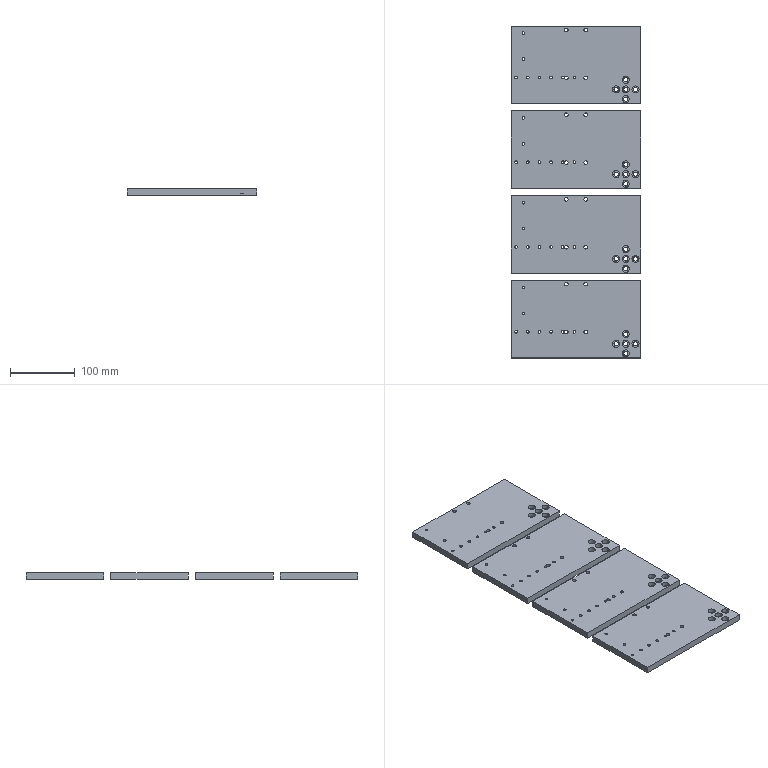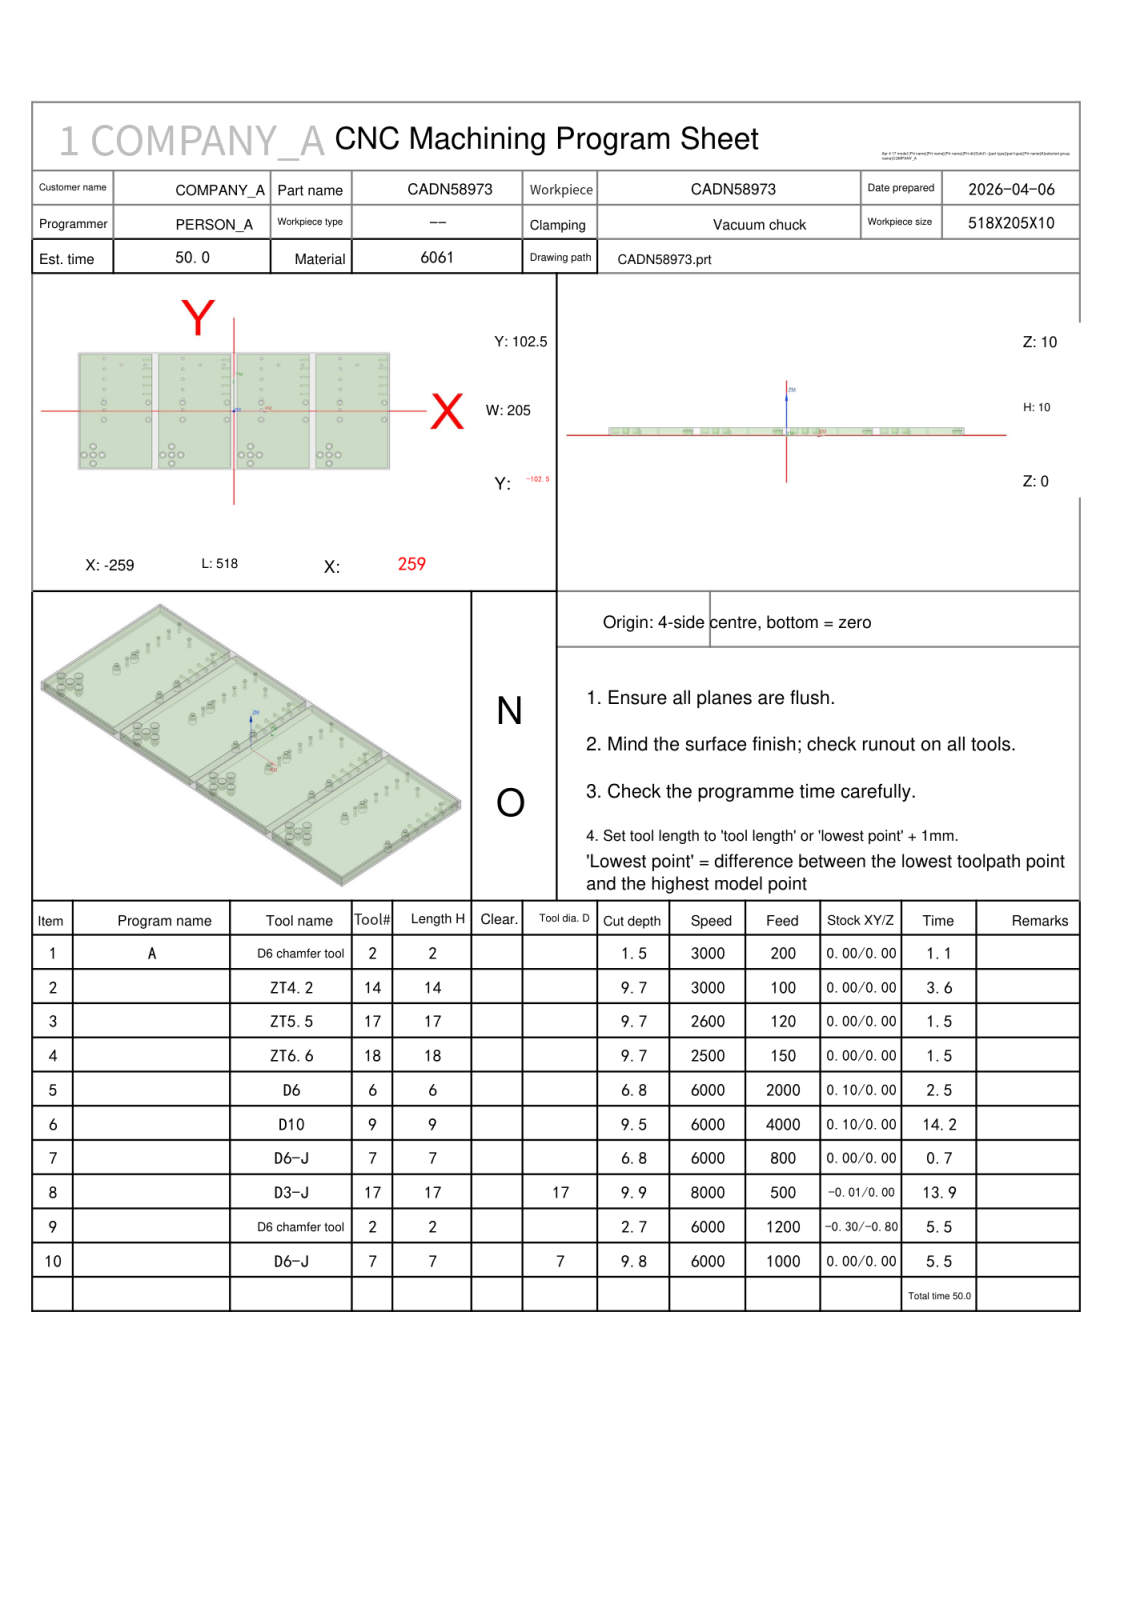NC program | NX | posted by the shop | part box 200 x 513 x 10 mm
Lines 9278 to 10035 of 10035:
N9 T02 M06
(D6 chamfer tool  D=6. R=0. H=02 ce=0.00 di=0.00)
G00 G90 G54 X258.628 Y.25 M03 S6000
G43 H02 Z30.
M08
Z12.099
G01 Z8.5 F1200.
G03 X258.328 Y.33 I-.3 J-.52
X257.808 Y.03 I0.0 J-.6
G01 X257.8 Y0.0
Y-100.
G02 X256.5 Y-101.3 I-1.3 J0.0
G01 X136.5
G02 X135.2 Y-100. I0.0 J1.3
G01 Y100.
G02 X136.5 Y101.3 I1.3 J0.0
G01 X256.5
G02 X257.8 Y100. I0.0 J-1.3
G01 Y0.0
X257.808 Y-.03
G03 X258.328 Y-.33 I.52 J.3
X258.628 Y-.25 I0.0 J.6
G01 Z12.099
G00 Z30.
X127.628 Y.25
Z12.099
G01 Z8.5
G03 X127.328 Y.33 I-.3 J-.52
X126.808 Y.03 I0.0 J-.6
G01 X126.8 Y0.0
Y-100.
G02 X125.5 Y-101.3 I-1.3 J0.0
G01 X5.5
G02 X4.2 Y-100. I0.0 J1.3
G01 Y100.
G02 X5.5 Y101.3 I1.3 J0.0
G01 X125.5
G02 X126.8 Y100. I0.0 J-1.3
G01 Y0.0
X126.808 Y-.03
G03 X127.328 Y-.33 I.52 J.3
X127.628 Y-.25 I0.0 J.6
G01 Z12.099
G00 Z30.
X-3.372 Y.25
Z12.099
G01 Z8.5
G03 X-3.672 Y.33 I-.3 J-.52
X-4.192 Y.03 I0.0 J-.6
G01 X-4.2 Y0.0
Y-100.
G02 X-5.5 Y-101.3 I-1.3 J0.0
G01 X-125.5
G02 X-126.8 Y-100. I0.0 J1.3
G01 Y100.
G02 X-125.5 Y101.3 I1.3 J0.0
G01 X-5.5
G02 X-4.2 Y100. I0.0 J-1.3
G01 Y0.0
X-4.192 Y-.03
G03 X-3.672 Y-.33 I.52 J.3
X-3.372 Y-.25 I0.0 J.6
G01 Z12.099
G00 Z30.
X-134.372 Y.25
Z12.099
G01 Z8.5
G03 X-134.672 Y.33 I-.3 J-.52
X-135.192 Y.03 I0.0 J-.6
G01 X-135.2 Y0.0
Y-100.
G02 X-136.5 Y-101.3 I-1.3 J0.0
G01 X-256.5
G02 X-257.8 Y-100. I0.0 J1.3
G01 Y100.
G02 X-256.5 Y101.3 I1.3 J0.0
G01 X-136.5
G02 X-135.2 Y100. I0.0 J-1.3
G01 Y0.0
X-135.192 Y-.03
G03 X-134.672 Y-.33 I.52 J.3
X-134.372 Y-.25 I0.0 J.6
G01 Z12.099
G00 Z30.
G00 G90 X-216. Y2.515 M03 S5000
Z30.
G98 G81 X-216. Y2.515 Z7.333 R13. F150.
Y20.515
Y38.515
Y56.515
Y74.515
Y92.515
X-187.5 Y81.264
X-147.5
X-85. Y2.515
Y20.515
Y38.515
Y56.515
Y74.515
Y92.515
X-56.5 Y81.264
X-16.5
X46. Y2.515
Y20.515
Y38.515
Y56.515
Y74.515
Y92.515
X74.5 Y81.264
X114.5
X177. Y92.515
X245.5 Y81.264
X205.5
X177. Y74.515
Y56.515
Y38.515
Y20.515
Y2.515
G80
G00 Z30.
G00 G90 X249.853 Y-15.065 M03 S6000
Z30.
Z9.1
G01 Z8.6 F600.
X249. Y-15.15
G03 X250.5 Y-16.65 I1.5 J0.0
X252.15 Y-15. I0.0 J1.65
X250.5 Y-13.35 I-1.65 J0.0
X248.85 Y-15. I0.0 J-1.65
X250.5 Y-16.65 I1.65 J0.0
X252. Y-15.15 I0.0 J1.5
G01 X251.147 Y-15.065
Z9.1
G00 Z30.
X249.853 Y14.935
Z9.1
G01 Z8.6
X249. Y14.85
G03 X250.5 Y13.35 I1.5 J0.0
X252.15 Y15. I0.0 J1.65
X250.5 Y16.65 I-1.65 J0.0
X248.85 Y15. I0.0 J-1.65
X250.5 Y13.35 I1.65 J0.0
X252. Y14.85 I0.0 J1.5
G01 X251.147 Y14.935
Z9.1
G00 Z30.
X175.853
Z9.1
G01 Z8.6
X175. Y14.85
G03 X176.5 Y13.35 I1.5 J0.0
X178.15 Y15. I0.0 J1.65
X176.5 Y16.65 I-1.65 J0.0
X174.85 Y15. I0.0 J-1.65
X176.5 Y13.35 I1.65 J0.0
X178. Y14.85 I0.0 J1.5
G01 X177.147 Y14.935
Z9.1
G00 Z30.
X175.853 Y-15.065
Z9.1
G01 Z8.6
X175. Y-15.15
G03 X176.5 Y-16.65 I1.5 J0.0
X178.15 Y-15. I0.0 J1.65
X176.5 Y-13.35 I-1.65 J0.0
X174.85 Y-15. I0.0 J-1.65
X176.5 Y-16.65 I1.65 J0.0
X178. Y-15.15 I0.0 J1.5
G01 X177.147 Y-15.065
Z9.1
G00 Z30.
X118.853
Z9.1
G01 Z8.6
X118. Y-15.15
G03 X119.5 Y-16.65 I1.5 J0.0
X121.15 Y-15. I0.0 J1.65
X119.5 Y-13.35 I-1.65 J0.0
X117.85 Y-15. I0.0 J-1.65
X119.5 Y-16.65 I1.65 J0.0
X121. Y-15.15 I0.0 J1.5
G01 X120.147 Y-15.065
Z9.1
G00 Z30.
X118.853 Y14.935
Z9.1
G01 Z8.6
X118. Y14.85
G03 X119.5 Y13.35 I1.5 J0.0
X121.15 Y15. I0.0 J1.65
X119.5 Y16.65 I-1.65 J0.0
X117.85 Y15. I0.0 J-1.65
X119.5 Y13.35 I1.65 J0.0
X121. Y14.85 I0.0 J1.5
G01 X120.147 Y14.935
Z9.1
G00 Z30.
X44.853
Z9.1
G01 Z8.6
X44. Y14.85
G03 X45.5 Y13.35 I1.5 J0.0
X47.15 Y15. I0.0 J1.65
X45.5 Y16.65 I-1.65 J0.0
X43.85 Y15. I0.0 J-1.65
X45.5 Y13.35 I1.65 J0.0
X47. Y14.85 I0.0 J1.5
G01 X46.147 Y14.935
Z9.1
G00 Z30.
X44.853 Y-15.065
Z9.1
G01 Z8.6
X44. Y-15.15
G03 X45.5 Y-16.65 I1.5 J0.0
X47.15 Y-15. I0.0 J1.65
X45.5 Y-13.35 I-1.65 J0.0
X43.85 Y-15. I0.0 J-1.65
X45.5 Y-16.65 I1.65 J0.0
X47. Y-15.15 I0.0 J1.5
G01 X46.147 Y-15.065
Z9.1
G00 Z30.
X-12.147
Z9.1
G01 Z8.6
X-13. Y-15.15
G03 X-11.5 Y-16.65 I1.5 J0.0
X-9.85 Y-15. I0.0 J1.65
X-11.5 Y-13.35 I-1.65 J0.0
X-13.15 Y-15. I0.0 J-1.65
X-11.5 Y-16.65 I1.65 J0.0
X-10. Y-15.15 I0.0 J1.5
G01 X-10.853 Y-15.065
Z9.1
G00 Z30.
X-12.147 Y14.935
Z9.1
G01 Z8.6
X-13. Y14.85
G03 X-11.5 Y13.35 I1.5 J0.0
X-9.85 Y15. I0.0 J1.65
X-11.5 Y16.65 I-1.65 J0.0
X-13.15 Y15. I0.0 J-1.65
X-11.5 Y13.35 I1.65 J0.0
X-10. Y14.85 I0.0 J1.5
G01 X-10.853 Y14.935
Z9.1
G00 Z30.
X-86.147
Z9.1
G01 Z8.6
X-87. Y14.85
G03 X-85.5 Y13.35 I1.5 J0.0
X-83.85 Y15. I0.0 J1.65
X-85.5 Y16.65 I-1.65 J0.0
X-87.15 Y15. I0.0 J-1.65
X-85.5 Y13.35 I1.65 J0.0
X-84. Y14.85 I0.0 J1.5
G01 X-84.853 Y14.935
Z9.1
G00 Z30.
X-86.147 Y-15.065
Z9.1
G01 Z8.6
X-87. Y-15.15
G03 X-85.5 Y-16.65 I1.5 J0.0
X-83.85 Y-15. I0.0 J1.65
X-85.5 Y-13.35 I-1.65 J0.0
X-87.15 Y-15. I0.0 J-1.65
X-85.5 Y-16.65 I1.65 J0.0
X-84. Y-15.15 I0.0 J1.5
G01 X-84.853 Y-15.065
Z9.1
G00 Z30.
X-143.147
Z9.1
G01 Z8.6
X-144. Y-15.15
G03 X-142.5 Y-16.65 I1.5 J0.0
X-140.85 Y-15. I0.0 J1.65
X-142.5 Y-13.35 I-1.65 J0.0
X-144.15 Y-15. I0.0 J-1.65
X-142.5 Y-16.65 I1.65 J0.0
X-141. Y-15.15 I0.0 J1.5
G01 X-141.853 Y-15.065
Z9.1
G00 Z30.
X-143.147 Y14.935
Z9.1
G01 Z8.6
X-144. Y14.85
G03 X-142.5 Y13.35 I1.5 J0.0
X-140.85 Y15. I0.0 J1.65
X-142.5 Y16.65 I-1.65 J0.0
X-144.15 Y15. I0.0 J-1.65
X-142.5 Y13.35 I1.65 J0.0
X-141. Y14.85 I0.0 J1.5
G01 X-141.853 Y14.935
Z9.1
G00 Z30.
X-217.147
Z9.1
G01 Z8.6
X-218. Y14.85
G03 X-216.5 Y13.35 I1.5 J0.0
X-214.85 Y15. I0.0 J1.65
X-216.5 Y16.65 I-1.65 J0.0
X-218.15 Y15. I0.0 J-1.65
X-216.5 Y13.35 I1.65 J0.0
X-215. Y14.85 I0.0 J1.5
G01 X-215.853 Y14.935
Z9.1
G00 Z30.
X-217.147 Y-15.065
Z9.1
G01 Z8.6
X-218. Y-15.15
G03 X-216.5 Y-16.65 I1.5 J0.0
X-214.85 Y-15. I0.0 J1.65
X-216.5 Y-13.35 I-1.65 J0.0
X-218.15 Y-15. I0.0 J-1.65
X-216.5 Y-16.65 I1.65 J0.0
X-215. Y-15.15 I0.0 J1.5
G01 X-215.853 Y-15.065
Z9.1
G00 Z30.
G00 G90 X170.795 Y-77.721 M03 S6000
Z30.
Z8.5
G01 Z8. F600.
X170.5 Y-77.8
G03 X173.5 Y-80.8 I3. J0.0
X177.3 Y-77. I0.0 J3.8
X173.5 Y-73.2 I-3.8 J0.0
X169.7 Y-77. I0.0 J-3.8
X173.5 Y-80.8 I3.8 J0.0
X176.5 Y-77.8 I0.0 J3.
G01 X176.205 Y-77.721
Z8.5
G00 Z30.
X155.795 Y-62.721
Z8.5
G01 Z8.
X155.5 Y-62.8
G03 X158.5 Y-65.8 I3. J0.0
X162.3 Y-62. I0.0 J3.8
X158.5 Y-58.2 I-3.8 J0.0
X154.7 Y-62. I0.0 J-3.8
X158.5 Y-65.8 I3.8 J0.0
X161.5 Y-62.8 I0.0 J3.
G01 X161.205 Y-62.721
Z8.5
G00 Z30.
X155.795 Y-77.721
Z8.5
G01 Z8.
X155.5 Y-77.8
G03 X158.5 Y-80.8 I3. J0.0
X162.3 Y-77. I0.0 J3.8
X158.5 Y-73.2 I-3.8 J0.0
X154.7 Y-77. I0.0 J-3.8
X158.5 Y-80.8 I3.8 J0.0
X161.5 Y-77.8 I0.0 J3.
G01 X161.205 Y-77.721
Z8.5
G00 Z30.
X155.795 Y-92.721
Z8.5
G01 Z8.
X155.5 Y-92.8
G03 X158.5 Y-95.8 I3. J0.0
X162.3 Y-92. I0.0 J3.8
X158.5 Y-88.2 I-3.8 J0.0
X154.7 Y-92. I0.0 J-3.8
X158.5 Y-95.8 I3.8 J0.0
X161.5 Y-92.8 I0.0 J3.
G01 X161.205 Y-92.721
Z8.5
G00 Z30.
X140.795 Y-77.721
Z8.5
G01 Z8.
X140.5 Y-77.8
G03 X143.5 Y-80.8 I3. J0.0
X147.3 Y-77. I0.0 J3.8
X143.5 Y-73.2 I-3.8 J0.0
X139.7 Y-77. I0.0 J-3.8
X143.5 Y-80.8 I3.8 J0.0
X146.5 Y-77.8 I0.0 J3.
G01 X146.205 Y-77.721
Z8.5
G00 Z30.
X39.795
Z8.5
G01 Z8.
X39.5 Y-77.8
G03 X42.5 Y-80.8 I3. J0.0
X46.3 Y-77. I0.0 J3.8
X42.5 Y-73.2 I-3.8 J0.0
X38.7 Y-77. I0.0 J-3.8
X42.5 Y-80.8 I3.8 J0.0
X45.5 Y-77.8 I0.0 J3.
G01 X45.205 Y-77.721
Z8.5
G00 Z30.
X24.795 Y-92.721
Z8.5
G01 Z8.
X24.5 Y-92.8
G03 X27.5 Y-95.8 I3. J0.0
X31.3 Y-92. I0.0 J3.8
X27.5 Y-88.2 I-3.8 J0.0
X23.7 Y-92. I0.0 J-3.8
X27.5 Y-95.8 I3.8 J0.0
X30.5 Y-92.8 I0.0 J3.
G01 X30.205 Y-92.721
Z8.5
G00 Z30.
X24.795 Y-77.721
Z8.5
G01 Z8.
X24.5 Y-77.8
G03 X27.5 Y-80.8 I3. J0.0
X31.3 Y-77. I0.0 J3.8
X27.5 Y-73.2 I-3.8 J0.0
X23.7 Y-77. I0.0 J-3.8
X27.5 Y-80.8 I3.8 J0.0
X30.5 Y-77.8 I0.0 J3.
G01 X30.205 Y-77.721
Z8.5
G00 Z30.
X24.795 Y-62.721
Z8.5
G01 Z8.
X24.5 Y-62.8
G03 X27.5 Y-65.8 I3. J0.0
X31.3 Y-62. I0.0 J3.8
X27.5 Y-58.2 I-3.8 J0.0
X23.7 Y-62. I0.0 J-3.8
X27.5 Y-65.8 I3.8 J0.0
X30.5 Y-62.8 I0.0 J3.
G01 X30.205 Y-62.721
Z8.5
G00 Z30.
X9.795 Y-77.721
Z8.5
G01 Z8.
X9.5 Y-77.8
G03 X12.5 Y-80.8 I3. J0.0
X16.3 Y-77. I0.0 J3.8
X12.5 Y-73.2 I-3.8 J0.0
X8.7 Y-77. I0.0 J-3.8
X12.5 Y-80.8 I3.8 J0.0
X15.5 Y-77.8 I0.0 J3.
G01 X15.205 Y-77.721
Z8.5
G00 Z30.
X-91.205
Z8.5
G01 Z8.
X-91.5 Y-77.8
G03 X-88.5 Y-80.8 I3. J0.0
X-84.7 Y-77. I0.0 J3.8
X-88.5 Y-73.2 I-3.8 J0.0
X-92.3 Y-77. I0.0 J-3.8
X-88.5 Y-80.8 I3.8 J0.0
X-85.5 Y-77.8 I0.0 J3.
G01 X-85.795 Y-77.721
Z8.5
G00 Z30.
X-106.205 Y-92.721
Z8.5
G01 Z8.
X-106.5 Y-92.8
G03 X-103.5 Y-95.8 I3. J0.0
X-99.7 Y-92. I0.0 J3.8
X-103.5 Y-88.2 I-3.8 J0.0
X-107.3 Y-92. I0.0 J-3.8
X-103.5 Y-95.8 I3.8 J0.0
X-100.5 Y-92.8 I0.0 J3.
G01 X-100.795 Y-92.721
Z8.5
G00 Z30.
X-106.205 Y-77.721
Z8.5
G01 Z8.
X-106.5 Y-77.8
G03 X-103.5 Y-80.8 I3. J0.0
X-99.7 Y-77. I0.0 J3.8
X-103.5 Y-73.2 I-3.8 J0.0
X-107.3 Y-77. I0.0 J-3.8
X-103.5 Y-80.8 I3.8 J0.0
X-100.5 Y-77.8 I0.0 J3.
G01 X-100.795 Y-77.721
Z8.5
G00 Z30.
X-106.205 Y-62.721
Z8.5
G01 Z8.
X-106.5 Y-62.8
G03 X-103.5 Y-65.8 I3. J0.0
X-99.7 Y-62. I0.0 J3.8
X-103.5 Y-58.2 I-3.8 J0.0
X-107.3 Y-62. I0.0 J-3.8
X-103.5 Y-65.8 I3.8 J0.0
X-100.5 Y-62.8 I0.0 J3.
G01 X-100.795 Y-62.721
Z8.5
G00 Z30.
X-121.205 Y-77.721
Z8.5
G01 Z8.
X-121.5 Y-77.8
G03 X-118.5 Y-80.8 I3. J0.0
X-114.7 Y-77. I0.0 J3.8
X-118.5 Y-73.2 I-3.8 J0.0
X-122.3 Y-77. I0.0 J-3.8
X-118.5 Y-80.8 I3.8 J0.0
X-115.5 Y-77.8 I0.0 J3.
G01 X-115.795 Y-77.721
Z8.5
G00 Z30.
X-222.205
Z8.5
G01 Z8.
X-222.5 Y-77.8
G03 X-219.5 Y-80.8 I3. J0.0
X-215.7 Y-77. I0.0 J3.8
X-219.5 Y-73.2 I-3.8 J0.0
X-223.3 Y-77. I0.0 J-3.8
X-219.5 Y-80.8 I3.8 J0.0
X-216.5 Y-77.8 I0.0 J3.
G01 X-216.795 Y-77.721
Z8.5
G00 Z30.
X-237.205
Z8.5
G01 Z8.
X-237.5 Y-77.8
G03 X-234.5 Y-80.8 I3. J0.0
X-230.7 Y-77. I0.0 J3.8
X-234.5 Y-73.2 I-3.8 J0.0
X-238.3 Y-77. I0.0 J-3.8
X-234.5 Y-80.8 I3.8 J0.0
X-231.5 Y-77.8 I0.0 J3.
G01 X-231.795 Y-77.721
Z8.5
G00 Z30.
X-237.205 Y-62.721
Z8.5
G01 Z8.
X-237.5 Y-62.8
G03 X-234.5 Y-65.8 I3. J0.0
X-230.7 Y-62. I0.0 J3.8
X-234.5 Y-58.2 I-3.8 J0.0
X-238.3 Y-62. I0.0 J-3.8
X-234.5 Y-65.8 I3.8 J0.0
X-231.5 Y-62.8 I0.0 J3.
G01 X-231.795 Y-62.721
Z8.5
G00 Z30.
X-252.205 Y-77.721
Z8.5
G01 Z8.
X-252.5 Y-77.8
G03 X-249.5 Y-80.8 I3. J0.0
X-245.7 Y-77. I0.0 J3.8
X-249.5 Y-73.2 I-3.8 J0.0
X-253.3 Y-77. I0.0 J-3.8
X-249.5 Y-80.8 I3.8 J0.0
X-246.5 Y-77.8 I0.0 J3.
G01 X-246.795 Y-77.721
Z8.5
G00 Z30.
X-237.205 Y-92.721
Z8.5
G01 Z8.
X-237.5 Y-92.8
G03 X-234.5 Y-95.8 I3. J0.0
X-230.7 Y-92. I0.0 J3.8
X-234.5 Y-88.2 I-3.8 J0.0
X-238.3 Y-92. I0.0 J-3.8
X-234.5 Y-95.8 I3.8 J0.0
X-231.5 Y-92.8 I0.0 J3.
G01 X-231.795 Y-92.721
Z8.5
G00 Z30.
G91 G28 Z0.0
M05
M09
G91 G28 Z0.0
M01
N10 T07 M06
(D6-J  D=6. R=0. H=07 ce=0.00 di=0.00)
G00 G90 G54 X-260.573 Y-101.017 M03 S6000
G43 H07 Z30.
M08
Z1.
G01 Z.5 F1000.
G41 D07
X-260.375 Y-100.992
G03 X-259.5 Y-100. I-.125 J.992
G01 Y100.
G02 X-256.5 Y103. I3. J0.0
G01 X-136.5
G02 X-133.5 Y100. I0.0 J-3.
G01 Y-100.
G02 X-136.5 Y-103. I-3. J0.0
G01 X-256.5
G02 X-259.5 Y-100. I0.0 J3.
G01 Y-99.5
G03 X-260.5 Y-98.5 I-1. J0.0
G01 G40 X-260.7
Z1.
G00 Z30.
X-129.573 Y-101.017
Z1.
G01 Z.5
G41 D07
X-129.375 Y-100.992
G03 X-128.5 Y-100. I-.125 J.992
G01 Y100.
G02 X-125.5 Y103. I3. J0.0
G01 X-5.5
G02 X-2.5 Y100. I0.0 J-3.
G01 Y-100.
G02 X-5.5 Y-103. I-3. J0.0
G01 X-125.5
G02 X-128.5 Y-100. I0.0 J3.
G01 Y-99.5
G03 X-129.5 Y-98.5 I-1. J0.0
G01 G40 X-129.7
Z1.
G00 Z30.
X1.427 Y-101.017
Z1.
G01 Z.5
G41 D07
X1.625 Y-100.992
G03 X2.5 Y-100. I-.125 J.992
G01 Y100.
G02 X5.5 Y103. I3. J0.0
G01 X125.5
G02 X128.5 Y100. I0.0 J-3.
G01 Y-100.
G02 X125.5 Y-103. I-3. J0.0
G01 X5.5
G02 X2.5 Y-100. I0.0 J3.
G01 Y-99.5
G03 X1.5 Y-98.5 I-1. J0.0
G01 G40 X1.3
Z1.
G00 Z30.
X260.573 Y101.017
Z1.
G01 Z.5
G41 D07
X260.375 Y100.992
G03 X259.5 Y100. I.125 J-.992
G01 Y-100.
G02 X256.5 Y-103. I-3. J0.0
G01 X136.5
G02 X133.5 Y-100. I0.0 J3.
G01 Y100.
G02 X136.5 Y103. I3. J0.0
G01 X256.5
G02 X259.5 Y100. I0.0 J-3.
G01 Y99.5
G03 X260.5 Y98.5 I1. J0.0
G01 G40 X260.7
Z1.
G00 Z30.
G00 G90 X-260.474 Y-101.005 M03 S6000
Z30.
Z.7
G01 Z.2 F1000.
G41 D07
X-260.375 Y-100.992
G03 X-259.5 Y-100. I-.125 J.992
G01 Y100.
G02 X-256.5 Y103. I3. J0.0
G01 X-136.5
G02 X-133.5 Y100. I0.0 J-3.
G01 Y-100.
G02 X-136.5 Y-103. I-3. J0.0
G01 X-256.5
G02 X-259.5 Y-100. I0.0 J3.
G01 Y-99.5
G03 X-260.5 Y-98.5 I-1. J0.0
G01 G40 X-260.6
Z.7
G00 Z30.
X-129.474 Y-101.005
Z.7
G01 Z.2
G41 D07
X-129.375 Y-100.992
G03 X-128.5 Y-100. I-.125 J.992
G01 Y100.
G02 X-125.5 Y103. I3. J0.0
G01 X-5.5
G02 X-2.5 Y100. I0.0 J-3.
G01 Y-100.
G02 X-5.5 Y-103. I-3. J0.0
G01 X-125.5
G02 X-128.5 Y-100. I0.0 J3.
G01 Y-99.5
G03 X-129.5 Y-98.5 I-1. J0.0
G01 G40 X-129.6
Z.7
G00 Z30.
X1.526 Y-101.005
Z.7
G01 Z.2
G41 D07
X1.625 Y-100.992
G03 X2.5 Y-100. I-.125 J.992
G01 Y100.
G02 X5.5 Y103. I3. J0.0
G01 X125.5
G02 X128.5 Y100. I0.0 J-3.
G01 Y-100.
G02 X125.5 Y-103. I-3. J0.0
G01 X5.5
G02 X2.5 Y-100. I0.0 J3.
G01 Y-99.5
G03 X1.5 Y-98.5 I-1. J0.0
G01 G40 X1.4
Z.7
G00 Z30.
X260.474 Y101.005
Z.7
G01 Z.2
G41 D07
X260.375 Y100.992
G03 X259.5 Y100. I.125 J-.992
G01 Y-100.
G02 X256.5 Y-103. I-3. J0.0
G01 X136.5
G02 X133.5 Y-100. I0.0 J3.
G01 Y100.
G02 X136.5 Y103. I3. J0.0
G01 X256.5
G02 X259.5 Y100. I0.0 J-3.
G01 Y99.5
G03 X260.5 Y98.5 I1. J0.0
G01 G40 X260.6
Z.7
G00 Z30.
M05
M09
G91 G28 Z0.0
G91 G28 Y0.0
M30
%